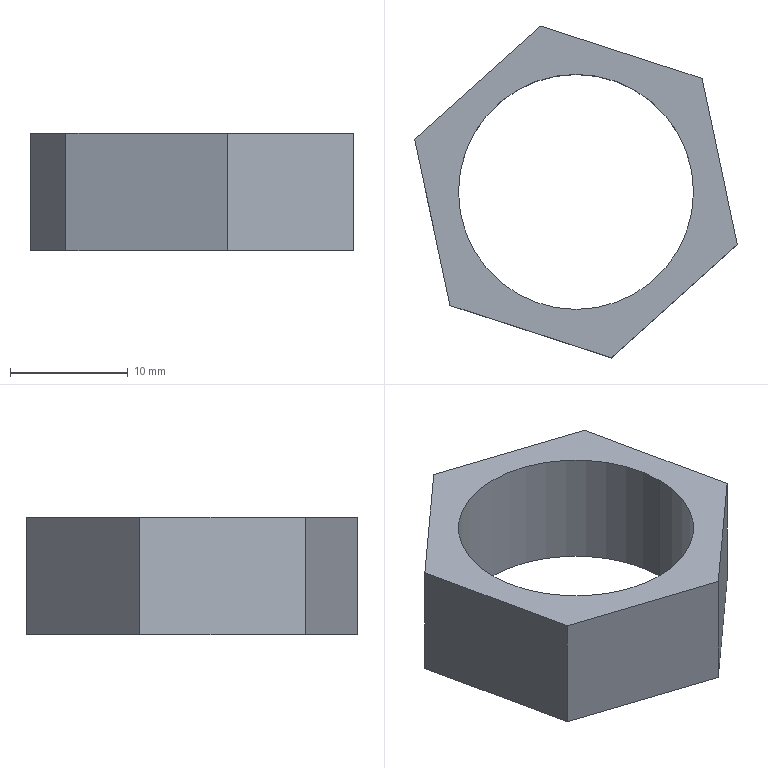Part | SolidWorks | features Extrusion 1 | 1 solid | 10 faces | box 27.456 x 28.236 x 10 mm | volume 2271 mm3 | plane 8 | cylinder 2 | commonest cylinder face diameters 20 x2
STEP:
#1=CARTESIAN_POINT('',(-10.,0.,10.));
#2=VERTEX_POINT('',#1);
#3=CARTESIAN_POINT('',(10.,0.,10.));
#4=VERTEX_POINT('',#3);
#5=CARTESIAN_POINT('',(0.,0.,10.));
#6=DIRECTION('',(0.,0.,1.));
#7=DIRECTION('',(1.,0.,0.));
#8=AXIS2_PLACEMENT_3D('',#5,#6,#7);
#9=CIRCLE('',#8,10.);
#10=EDGE_CURVE('',#2,#4,#9,.T.);
#11=ORIENTED_EDGE('',*,*,#10,.T.);
#12=CARTESIAN_POINT('',(10.,0.,0.));
#13=VERTEX_POINT('',#12);
#14=CARTESIAN_POINT('',(10.,0.,10.));
#15=DIRECTION('',(0.,0.,-1.));
#16=VECTOR('',#15,1000.);
#17=LINE('',#14,#16);
#18=EDGE_CURVE('',#4,#13,#17,.T.);
#19=ORIENTED_EDGE('',*,*,#18,.T.);
#20=CARTESIAN_POINT('',(-10.,0.,0.));
#21=VERTEX_POINT('',#20);
#22=CARTESIAN_POINT('',(0.,0.,0.));
#23=DIRECTION('',(0.,0.,1.));
#24=DIRECTION('',(1.,0.,0.));
#25=AXIS2_PLACEMENT_3D('',#22,#23,#24);
#26=CIRCLE('',#25,10.);
#27=EDGE_CURVE('',#21,#13,#26,.T.);
#28=ORIENTED_EDGE('',*,*,#27,.F.);
#29=CARTESIAN_POINT('',(-10.,0.,10.));
#30=DIRECTION('',(0.,0.,-1.));
#31=VECTOR('',#30,1000.);
#32=LINE('',#29,#31);
#33=EDGE_CURVE('',#2,#21,#32,.T.);
#34=ORIENTED_EDGE('',*,*,#33,.F.);
#35=EDGE_LOOP('',(#11,#19,#28,#34));
#36=FACE_OUTER_BOUND('',#35,.T.);
#37=CARTESIAN_POINT('',(0.,0.,10.));
#38=DIRECTION('',(0.,0.,-1.));
#39=DIRECTION('',(-1.,0.,0.));
#40=AXIS2_PLACEMENT_3D('',#37,#38,#39);
#41=CYLINDRICAL_SURFACE('',#40,10.);
#42=ADVANCED_FACE('',(#36),#41,.F.);
#43=CARTESIAN_POINT('',(13.728,-4.458,10.));
#44=VERTEX_POINT('',#43);
#45=CARTESIAN_POINT('',(10.725,9.66,10.));
#46=VERTEX_POINT('',#45);
#47=CARTESIAN_POINT('',(13.728,-4.458,10.));
#48=DIRECTION('',(-0.2081,0.9781,0.));
#49=VECTOR('',#48,1000.);
#50=LINE('',#47,#49);
#51=EDGE_CURVE('',#44,#46,#50,.T.);
#52=ORIENTED_EDGE('',*,*,#51,.T.);
#53=CARTESIAN_POINT('',(-3.003,14.118,10.));
#54=VERTEX_POINT('',#53);
#55=CARTESIAN_POINT('',(10.725,9.66,10.));
#56=DIRECTION('',(-0.9511,0.3089,0.));
#57=VECTOR('',#56,1000.);
#58=LINE('',#55,#57);
#59=EDGE_CURVE('',#46,#54,#58,.T.);
#60=ORIENTED_EDGE('',*,*,#59,.T.);
#61=CARTESIAN_POINT('',(-13.728,4.458,10.));
#62=VERTEX_POINT('',#61);
#63=CARTESIAN_POINT('',(-3.003,14.118,10.));
#64=DIRECTION('',(-0.743,-0.6693,0.));
#65=VECTOR('',#64,1000.);
#66=LINE('',#63,#65);
#67=EDGE_CURVE('',#54,#62,#66,.T.);
#68=ORIENTED_EDGE('',*,*,#67,.T.);
#69=CARTESIAN_POINT('',(-10.725,-9.66,10.));
#70=VERTEX_POINT('',#69);
#71=CARTESIAN_POINT('',(-13.728,4.458,10.));
#72=DIRECTION('',(0.2081,-0.9781,0.));
#73=VECTOR('',#72,1000.);
#74=LINE('',#71,#73);
#75=EDGE_CURVE('',#62,#70,#74,.T.);
#76=ORIENTED_EDGE('',*,*,#75,.T.);
#77=CARTESIAN_POINT('',(3.003,-14.118,10.));
#78=VERTEX_POINT('',#77);
#79=CARTESIAN_POINT('',(-10.725,-9.66,10.));
#80=DIRECTION('',(0.9511,-0.3089,0.));
#81=VECTOR('',#80,1000.);
#82=LINE('',#79,#81);
#83=EDGE_CURVE('',#70,#78,#82,.T.);
#84=ORIENTED_EDGE('',*,*,#83,.T.);
#85=CARTESIAN_POINT('',(3.003,-14.118,10.));
#86=DIRECTION('',(0.743,0.6693,0.));
#87=VECTOR('',#86,1000.);
#88=LINE('',#85,#87);
#89=EDGE_CURVE('',#78,#44,#88,.T.);
#90=ORIENTED_EDGE('',*,*,#89,.T.);
#91=EDGE_LOOP('',(#52,#60,#68,#76,#84,#90));
#92=FACE_OUTER_BOUND('',#91,.T.);
#93=ORIENTED_EDGE('',*,*,#10,.F.);
#94=CARTESIAN_POINT('',(0.,0.,10.));
#95=DIRECTION('',(0.,0.,1.));
#96=DIRECTION('',(1.,0.,0.));
#97=AXIS2_PLACEMENT_3D('',#94,#95,#96);
#98=CIRCLE('',#97,10.);
#99=EDGE_CURVE('',#4,#2,#98,.T.);
#100=ORIENTED_EDGE('',*,*,#99,.F.);
#101=EDGE_LOOP('',(#93,#100));
#102=FACE_BOUND('',#101,.T.);
#103=CARTESIAN_POINT('',(0.,0.,10.));
#104=DIRECTION('',(0.,0.,1.));
#105=DIRECTION('',(1.,0.,0.));
#106=AXIS2_PLACEMENT_3D('',#103,#104,#105);
#107=PLANE('',#106);
#108=ADVANCED_FACE('',(#92,#102),#107,.T.);
#109=CARTESIAN_POINT('',(13.728,-4.458,0.));
#110=VERTEX_POINT('',#109);
#111=CARTESIAN_POINT('',(10.725,9.66,0.));
#112=VERTEX_POINT('',#111);
#113=CARTESIAN_POINT('',(13.728,-4.458,0.));
#114=DIRECTION('',(-0.2081,0.9781,0.));
#115=VECTOR('',#114,1000.);
#116=LINE('',#113,#115);
#117=EDGE_CURVE('',#110,#112,#116,.T.);
#118=ORIENTED_EDGE('',*,*,#117,.F.);
#119=CARTESIAN_POINT('',(3.003,-14.118,0.));
#120=VERTEX_POINT('',#119);
#121=CARTESIAN_POINT('',(3.003,-14.118,0.));
#122=DIRECTION('',(0.743,0.6693,0.));
#123=VECTOR('',#122,1000.);
#124=LINE('',#121,#123);
#125=EDGE_CURVE('',#120,#110,#124,.T.);
#126=ORIENTED_EDGE('',*,*,#125,.F.);
#127=CARTESIAN_POINT('',(-10.725,-9.66,0.));
#128=VERTEX_POINT('',#127);
#129=CARTESIAN_POINT('',(-10.725,-9.66,0.));
#130=DIRECTION('',(0.9511,-0.3089,0.));
#131=VECTOR('',#130,1000.);
#132=LINE('',#129,#131);
#133=EDGE_CURVE('',#128,#120,#132,.T.);
#134=ORIENTED_EDGE('',*,*,#133,.F.);
#135=CARTESIAN_POINT('',(-13.728,4.458,0.));
#136=VERTEX_POINT('',#135);
#137=CARTESIAN_POINT('',(-13.728,4.458,0.));
#138=DIRECTION('',(0.2081,-0.9781,0.));
#139=VECTOR('',#138,1000.);
#140=LINE('',#137,#139);
#141=EDGE_CURVE('',#136,#128,#140,.T.);
#142=ORIENTED_EDGE('',*,*,#141,.F.);
#143=CARTESIAN_POINT('',(-3.003,14.118,0.));
#144=VERTEX_POINT('',#143);
#145=CARTESIAN_POINT('',(-3.003,14.118,0.));
#146=DIRECTION('',(-0.743,-0.6693,0.));
#147=VECTOR('',#146,1000.);
#148=LINE('',#145,#147);
#149=EDGE_CURVE('',#144,#136,#148,.T.);
#150=ORIENTED_EDGE('',*,*,#149,.F.);
#151=CARTESIAN_POINT('',(10.725,9.66,0.));
#152=DIRECTION('',(-0.9511,0.3089,0.));
#153=VECTOR('',#152,1000.);
#154=LINE('',#151,#153);
#155=EDGE_CURVE('',#112,#144,#154,.T.);
#156=ORIENTED_EDGE('',*,*,#155,.F.);
#157=EDGE_LOOP('',(#118,#126,#134,#142,#150,#156));
#158=FACE_OUTER_BOUND('',#157,.T.);
#159=ORIENTED_EDGE('',*,*,#27,.T.);
#160=CARTESIAN_POINT('',(0.,0.,0.));
#161=DIRECTION('',(0.,0.,1.));
#162=DIRECTION('',(1.,0.,0.));
#163=AXIS2_PLACEMENT_3D('',#160,#161,#162);
#164=CIRCLE('',#163,10.);
#165=EDGE_CURVE('',#13,#21,#164,.T.);
#166=ORIENTED_EDGE('',*,*,#165,.T.);
#167=EDGE_LOOP('',(#159,#166));
#168=FACE_BOUND('',#167,.T.);
#169=CARTESIAN_POINT('',(0.,0.,0.));
#170=DIRECTION('',(0.,0.,1.));
#171=DIRECTION('',(1.,0.,0.));
#172=AXIS2_PLACEMENT_3D('',#169,#170,#171);
#173=PLANE('',#172);
#174=ADVANCED_FACE('',(#158,#168),#173,.F.);
#175=ORIENTED_EDGE('',*,*,#117,.T.);
#176=CARTESIAN_POINT('',(10.725,9.66,10.));
#177=DIRECTION('',(0.,0.,-1.));
#178=VECTOR('',#177,1000.);
#179=LINE('',#176,#178);
#180=EDGE_CURVE('',#46,#112,#179,.T.);
#181=ORIENTED_EDGE('',*,*,#180,.F.);
#182=ORIENTED_EDGE('',*,*,#51,.F.);
#183=CARTESIAN_POINT('',(13.728,-4.458,10.));
#184=DIRECTION('',(0.,0.,-1.));
#185=VECTOR('',#184,1000.);
#186=LINE('',#183,#185);
#187=EDGE_CURVE('',#44,#110,#186,.T.);
#188=ORIENTED_EDGE('',*,*,#187,.T.);
#189=EDGE_LOOP('',(#175,#181,#182,#188));
#190=FACE_OUTER_BOUND('',#189,.T.);
#191=CARTESIAN_POINT('',(13.728,-4.458,10.));
#192=DIRECTION('',(-0.9781,-0.2081,0.));
#193=DIRECTION('',(0.2081,-0.9781,0.));
#194=AXIS2_PLACEMENT_3D('',#191,#192,#193);
#195=PLANE('',#194);
#196=ADVANCED_FACE('',(#190),#195,.F.);
#197=ORIENTED_EDGE('',*,*,#155,.T.);
#198=CARTESIAN_POINT('',(-3.003,14.118,10.));
#199=DIRECTION('',(0.,0.,-1.));
#200=VECTOR('',#199,1000.);
#201=LINE('',#198,#200);
#202=EDGE_CURVE('',#54,#144,#201,.T.);
#203=ORIENTED_EDGE('',*,*,#202,.F.);
#204=ORIENTED_EDGE('',*,*,#59,.F.);
#205=ORIENTED_EDGE('',*,*,#180,.T.);
#206=EDGE_LOOP('',(#197,#203,#204,#205));
#207=FACE_OUTER_BOUND('',#206,.T.);
#208=CARTESIAN_POINT('',(10.725,9.66,10.));
#209=DIRECTION('',(-0.3089,-0.9511,0.));
#210=DIRECTION('',(0.9511,-0.3089,0.));
#211=AXIS2_PLACEMENT_3D('',#208,#209,#210);
#212=PLANE('',#211);
#213=ADVANCED_FACE('',(#207),#212,.F.);
#214=ORIENTED_EDGE('',*,*,#149,.T.);
#215=CARTESIAN_POINT('',(-13.728,4.458,10.));
#216=DIRECTION('',(0.,0.,-1.));
#217=VECTOR('',#216,1000.);
#218=LINE('',#215,#217);
#219=EDGE_CURVE('',#62,#136,#218,.T.);
#220=ORIENTED_EDGE('',*,*,#219,.F.);
#221=ORIENTED_EDGE('',*,*,#67,.F.);
#222=ORIENTED_EDGE('',*,*,#202,.T.);
#223=EDGE_LOOP('',(#214,#220,#221,#222));
#224=FACE_OUTER_BOUND('',#223,.T.);
#225=CARTESIAN_POINT('',(-3.003,14.118,10.));
#226=DIRECTION('',(0.6693,-0.743,0.));
#227=DIRECTION('',(0.743,0.6693,0.));
#228=AXIS2_PLACEMENT_3D('',#225,#226,#227);
#229=PLANE('',#228);
#230=ADVANCED_FACE('',(#224),#229,.F.);
#231=ORIENTED_EDGE('',*,*,#141,.T.);
#232=CARTESIAN_POINT('',(-10.725,-9.66,10.));
#233=DIRECTION('',(0.,0.,-1.));
#234=VECTOR('',#233,1000.);
#235=LINE('',#232,#234);
#236=EDGE_CURVE('',#70,#128,#235,.T.);
#237=ORIENTED_EDGE('',*,*,#236,.F.);
#238=ORIENTED_EDGE('',*,*,#75,.F.);
#239=ORIENTED_EDGE('',*,*,#219,.T.);
#240=EDGE_LOOP('',(#231,#237,#238,#239));
#241=FACE_OUTER_BOUND('',#240,.T.);
#242=CARTESIAN_POINT('',(-13.728,4.458,10.));
#243=DIRECTION('',(0.9781,0.2081,0.));
#244=DIRECTION('',(-0.2081,0.9781,0.));
#245=AXIS2_PLACEMENT_3D('',#242,#243,#244);
#246=PLANE('',#245);
#247=ADVANCED_FACE('',(#241),#246,.F.);
#248=ORIENTED_EDGE('',*,*,#133,.T.);
#249=CARTESIAN_POINT('',(3.003,-14.118,10.));
#250=DIRECTION('',(0.,0.,-1.));
#251=VECTOR('',#250,1000.);
#252=LINE('',#249,#251);
#253=EDGE_CURVE('',#78,#120,#252,.T.);
#254=ORIENTED_EDGE('',*,*,#253,.F.);
#255=ORIENTED_EDGE('',*,*,#83,.F.);
#256=ORIENTED_EDGE('',*,*,#236,.T.);
#257=EDGE_LOOP('',(#248,#254,#255,#256));
#258=FACE_OUTER_BOUND('',#257,.T.);
#259=CARTESIAN_POINT('',(-10.725,-9.66,10.));
#260=DIRECTION('',(0.3089,0.9511,0.));
#261=DIRECTION('',(-0.9511,0.3089,0.));
#262=AXIS2_PLACEMENT_3D('',#259,#260,#261);
#263=PLANE('',#262);
#264=ADVANCED_FACE('',(#258),#263,.F.);
#265=ORIENTED_EDGE('',*,*,#125,.T.);
#266=ORIENTED_EDGE('',*,*,#187,.F.);
#267=ORIENTED_EDGE('',*,*,#89,.F.);
#268=ORIENTED_EDGE('',*,*,#253,.T.);
#269=EDGE_LOOP('',(#265,#266,#267,#268));
#270=FACE_OUTER_BOUND('',#269,.T.);
#271=CARTESIAN_POINT('',(3.003,-14.118,10.));
#272=DIRECTION('',(-0.6693,0.743,0.));
#273=DIRECTION('',(-0.743,-0.6693,0.));
#274=AXIS2_PLACEMENT_3D('',#271,#272,#273);
#275=PLANE('',#274);
#276=ADVANCED_FACE('',(#270),#275,.F.);
#277=ORIENTED_EDGE('',*,*,#18,.F.);
#278=ORIENTED_EDGE('',*,*,#99,.T.);
#279=ORIENTED_EDGE('',*,*,#33,.T.);
#280=ORIENTED_EDGE('',*,*,#165,.F.);
#281=EDGE_LOOP('',(#277,#278,#279,#280));
#282=FACE_OUTER_BOUND('',#281,.T.);
#283=CARTESIAN_POINT('',(0.,0.,10.));
#284=DIRECTION('',(0.,0.,-1.));
#285=DIRECTION('',(-1.,0.,0.));
#286=AXIS2_PLACEMENT_3D('',#283,#284,#285);
#287=CYLINDRICAL_SURFACE('',#286,10.);
#288=ADVANCED_FACE('',(#282),#287,.F.);
#289=CLOSED_SHELL('',(#42,#108,#174,#196,#213,#230,#247,#264,#276,#288));
#290=MANIFOLD_SOLID_BREP('',#289);
#291=CARTESIAN_POINT('',(0.,0.,0.));
#292=DIRECTION('',(0.,0.,1.));
#293=DIRECTION('',(1.,0.,0.));
#294=AXIS2_PLACEMENT_3D('',#291,#292,#293);
#295=(LENGTH_UNIT()NAMED_UNIT(*)SI_UNIT(.MILLI.,.METRE.));
#296=UNCERTAINTY_MEASURE_WITH_UNIT(LENGTH_MEASURE(0.00001),#295,'','');
#297=(NAMED_UNIT(*)PLANE_ANGLE_UNIT()SI_UNIT($,.RADIAN.));
#298=(NAMED_UNIT(*)SI_UNIT($,.STERADIAN.)SOLID_ANGLE_UNIT());
#299=(GEOMETRIC_REPRESENTATION_CONTEXT(3)GLOBAL_UNCERTAINTY_ASSIGNED_CONTEXT((#296))GLOBAL_UNIT_ASSIGNED_CONTEXT((#295,#297,#298))REPRESENTATION_CONTEXT('',''));
#300=ADVANCED_BREP_SHAPE_REPRESENTATION('',(#290,#294),#299);